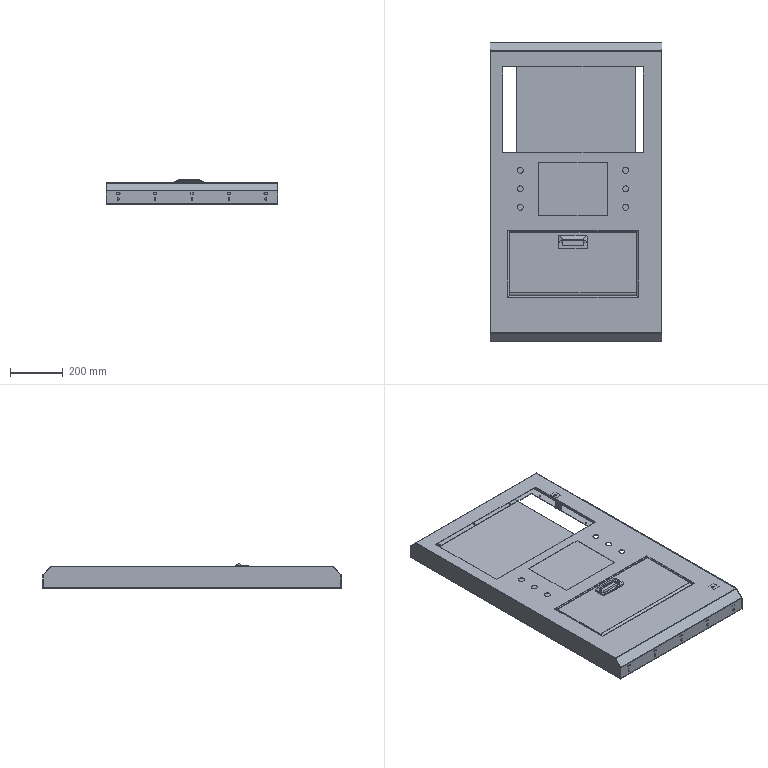Part | NX | features BREP 31 | 42 solids | 1288 faces | box 650 x 1132 x 95 mm | volume 2734251 mm3 | plane 641 | cylinder 475 | cone 144 | spline 20 | sphere 4 | torus 4 | commonest cylinder face diameters 6 x93 8 x57 4.2 x48 4 x33 3.3 x28 4.5 x24